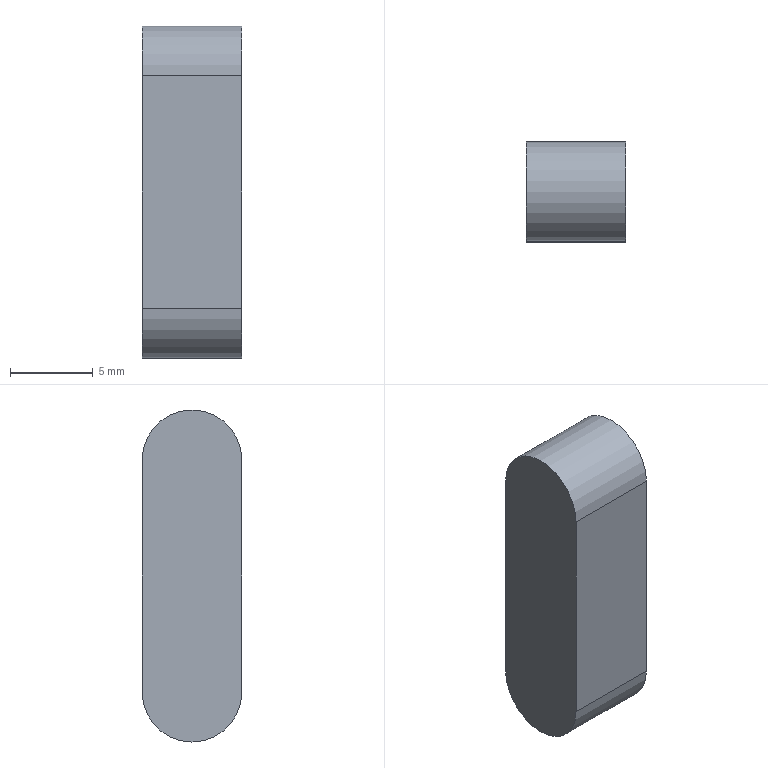Part | STEP file | KESS6-20 | 1 solid | 6 faces | box 6 x 6 x 20 mm | volume 673.646 mm3 | plane 4 | cylinder 2 | commonest cylinder face diameters 6 x2
STEP:
#1=CARTESIAN_POINT('',(6.,-3.,-19.));
#2=VERTEX_POINT('',#1);
#3=CARTESIAN_POINT('',(6.,-3.,-5.));
#4=VERTEX_POINT('',#3);
#5=CARTESIAN_POINT('',(6.,-3.,-19.));
#6=DIRECTION('',(0.,0.,1.));
#7=VECTOR('',#6,1000.);
#8=LINE('',#5,#7);
#9=EDGE_CURVE('',#2,#4,#8,.T.);
#10=ORIENTED_EDGE('',*,*,#9,.T.);
#11=CARTESIAN_POINT('',(0.,-3.,-5.));
#12=VERTEX_POINT('',#11);
#13=CARTESIAN_POINT('',(0.,-3.,-5.));
#14=DIRECTION('',(1.,0.,0.));
#15=VECTOR('',#14,1000.);
#16=LINE('',#13,#15);
#17=EDGE_CURVE('',#12,#4,#16,.T.);
#18=ORIENTED_EDGE('',*,*,#17,.F.);
#19=CARTESIAN_POINT('',(0.,-3.,-19.));
#20=VERTEX_POINT('',#19);
#21=CARTESIAN_POINT('',(0.,-3.,-19.));
#22=DIRECTION('',(0.,0.,1.));
#23=VECTOR('',#22,1000.);
#24=LINE('',#21,#23);
#25=EDGE_CURVE('',#20,#12,#24,.T.);
#26=ORIENTED_EDGE('',*,*,#25,.F.);
#27=CARTESIAN_POINT('',(0.,-3.,-19.));
#28=DIRECTION('',(1.,0.,0.));
#29=VECTOR('',#28,1000.);
#30=LINE('',#27,#29);
#31=EDGE_CURVE('',#20,#2,#30,.T.);
#32=ORIENTED_EDGE('',*,*,#31,.T.);
#33=EDGE_LOOP('',(#10,#18,#26,#32));
#34=FACE_OUTER_BOUND('',#33,.T.);
#35=CARTESIAN_POINT('',(0.,-3.,-19.));
#36=DIRECTION('',(0.,1.,0.));
#37=DIRECTION('',(-1.,0.,0.));
#38=AXIS2_PLACEMENT_3D('',#35,#36,#37);
#39=PLANE('',#38);
#40=ADVANCED_FACE('',(#34),#39,.F.);
#41=CARTESIAN_POINT('',(6.,3.,-5.));
#42=VERTEX_POINT('',#41);
#43=CARTESIAN_POINT('',(6.,0.,-5.));
#44=DIRECTION('',(-1.,0.,0.));
#45=DIRECTION('',(0.,-1.,0.));
#46=AXIS2_PLACEMENT_3D('',#43,#44,#45);
#47=CIRCLE('',#46,3.);
#48=EDGE_CURVE('',#4,#42,#47,.T.);
#49=ORIENTED_EDGE('',*,*,#48,.T.);
#50=CARTESIAN_POINT('',(0.,3.,-5.));
#51=VERTEX_POINT('',#50);
#52=CARTESIAN_POINT('',(0.,3.,-5.));
#53=DIRECTION('',(1.,0.,0.));
#54=VECTOR('',#53,1000.);
#55=LINE('',#52,#54);
#56=EDGE_CURVE('',#51,#42,#55,.T.);
#57=ORIENTED_EDGE('',*,*,#56,.F.);
#58=CARTESIAN_POINT('',(0.,0.,-5.));
#59=DIRECTION('',(-1.,0.,0.));
#60=DIRECTION('',(0.,-1.,0.));
#61=AXIS2_PLACEMENT_3D('',#58,#59,#60);
#62=CIRCLE('',#61,3.);
#63=EDGE_CURVE('',#12,#51,#62,.T.);
#64=ORIENTED_EDGE('',*,*,#63,.F.);
#65=ORIENTED_EDGE('',*,*,#17,.T.);
#66=EDGE_LOOP('',(#49,#57,#64,#65));
#67=FACE_OUTER_BOUND('',#66,.T.);
#68=CARTESIAN_POINT('',(0.,0.,-5.));
#69=DIRECTION('',(1.,0.,0.));
#70=DIRECTION('',(0.,1.,0.));
#71=AXIS2_PLACEMENT_3D('',#68,#69,#70);
#72=CYLINDRICAL_SURFACE('',#71,3.);
#73=ADVANCED_FACE('',(#67),#72,.T.);
#74=CARTESIAN_POINT('',(6.,3.,-19.));
#75=VERTEX_POINT('',#74);
#76=CARTESIAN_POINT('',(6.,3.,-5.));
#77=DIRECTION('',(0.,0.,-1.));
#78=VECTOR('',#77,1000.);
#79=LINE('',#76,#78);
#80=EDGE_CURVE('',#42,#75,#79,.T.);
#81=ORIENTED_EDGE('',*,*,#80,.T.);
#82=CARTESIAN_POINT('',(0.,3.,-19.));
#83=VERTEX_POINT('',#82);
#84=CARTESIAN_POINT('',(0.,3.,-19.));
#85=DIRECTION('',(1.,0.,0.));
#86=VECTOR('',#85,1000.);
#87=LINE('',#84,#86);
#88=EDGE_CURVE('',#83,#75,#87,.T.);
#89=ORIENTED_EDGE('',*,*,#88,.F.);
#90=CARTESIAN_POINT('',(0.,3.,-5.));
#91=DIRECTION('',(0.,0.,-1.));
#92=VECTOR('',#91,1000.);
#93=LINE('',#90,#92);
#94=EDGE_CURVE('',#51,#83,#93,.T.);
#95=ORIENTED_EDGE('',*,*,#94,.F.);
#96=ORIENTED_EDGE('',*,*,#56,.T.);
#97=EDGE_LOOP('',(#81,#89,#95,#96));
#98=FACE_OUTER_BOUND('',#97,.T.);
#99=CARTESIAN_POINT('',(0.,3.,-5.));
#100=DIRECTION('',(0.,-1.,0.));
#101=DIRECTION('',(1.,0.,0.));
#102=AXIS2_PLACEMENT_3D('',#99,#100,#101);
#103=PLANE('',#102);
#104=ADVANCED_FACE('',(#98),#103,.F.);
#105=CARTESIAN_POINT('',(6.,0.,-19.));
#106=DIRECTION('',(-1.,0.,0.));
#107=DIRECTION('',(0.,-1.,0.));
#108=AXIS2_PLACEMENT_3D('',#105,#106,#107);
#109=CIRCLE('',#108,3.);
#110=EDGE_CURVE('',#75,#2,#109,.T.);
#111=ORIENTED_EDGE('',*,*,#110,.T.);
#112=ORIENTED_EDGE('',*,*,#31,.F.);
#113=CARTESIAN_POINT('',(0.,0.,-19.));
#114=DIRECTION('',(-1.,0.,0.));
#115=DIRECTION('',(0.,-1.,0.));
#116=AXIS2_PLACEMENT_3D('',#113,#114,#115);
#117=CIRCLE('',#116,3.);
#118=EDGE_CURVE('',#83,#20,#117,.T.);
#119=ORIENTED_EDGE('',*,*,#118,.F.);
#120=ORIENTED_EDGE('',*,*,#88,.T.);
#121=EDGE_LOOP('',(#111,#112,#119,#120));
#122=FACE_OUTER_BOUND('',#121,.T.);
#123=CARTESIAN_POINT('',(0.,0.,-19.));
#124=DIRECTION('',(1.,0.,0.));
#125=DIRECTION('',(0.,1.,0.));
#126=AXIS2_PLACEMENT_3D('',#123,#124,#125);
#127=CYLINDRICAL_SURFACE('',#126,3.);
#128=ADVANCED_FACE('',(#122),#127,.T.);
#129=ORIENTED_EDGE('',*,*,#25,.T.);
#130=ORIENTED_EDGE('',*,*,#63,.T.);
#131=ORIENTED_EDGE('',*,*,#94,.T.);
#132=ORIENTED_EDGE('',*,*,#118,.T.);
#133=EDGE_LOOP('',(#129,#130,#131,#132));
#134=FACE_OUTER_BOUND('',#133,.T.);
#135=CARTESIAN_POINT('',(0.,0.,-5.));
#136=DIRECTION('',(-1.,0.,0.));
#137=DIRECTION('',(0.,-1.,0.));
#138=AXIS2_PLACEMENT_3D('',#135,#136,#137);
#139=PLANE('',#138);
#140=ADVANCED_FACE('',(#134),#139,.T.);
#141=ORIENTED_EDGE('',*,*,#9,.F.);
#142=ORIENTED_EDGE('',*,*,#110,.F.);
#143=ORIENTED_EDGE('',*,*,#80,.F.);
#144=ORIENTED_EDGE('',*,*,#48,.F.);
#145=EDGE_LOOP('',(#141,#142,#143,#144));
#146=FACE_OUTER_BOUND('',#145,.T.);
#147=CARTESIAN_POINT('',(6.,0.,-5.));
#148=DIRECTION('',(-1.,0.,0.));
#149=DIRECTION('',(0.,-1.,0.));
#150=AXIS2_PLACEMENT_3D('',#147,#148,#149);
#151=PLANE('',#150);
#152=ADVANCED_FACE('',(#146),#151,.F.);
#153=CLOSED_SHELL('',(#40,#73,#104,#128,#140,#152));
#154=MANIFOLD_SOLID_BREP('',#153);
#155=CARTESIAN_POINT('',(0.,0.,0.));
#156=DIRECTION('',(0.,0.,1.));
#157=DIRECTION('',(1.,0.,0.));
#158=AXIS2_PLACEMENT_3D('',#155,#156,#157);
#159=(LENGTH_UNIT()NAMED_UNIT(*)SI_UNIT(.MILLI.,.METRE.));
#160=UNCERTAINTY_MEASURE_WITH_UNIT(LENGTH_MEASURE(0.00001),#159,'','');
#161=(NAMED_UNIT(*)PLANE_ANGLE_UNIT()SI_UNIT($,.RADIAN.));
#162=(NAMED_UNIT(*)SI_UNIT($,.STERADIAN.)SOLID_ANGLE_UNIT());
#163=(GEOMETRIC_REPRESENTATION_CONTEXT(3)GLOBAL_UNCERTAINTY_ASSIGNED_CONTEXT((#160))GLOBAL_UNIT_ASSIGNED_CONTEXT((#159,#161,#162))REPRESENTATION_CONTEXT('',''));
#164=ADVANCED_BREP_SHAPE_REPRESENTATION('',(#154,#158),#163);